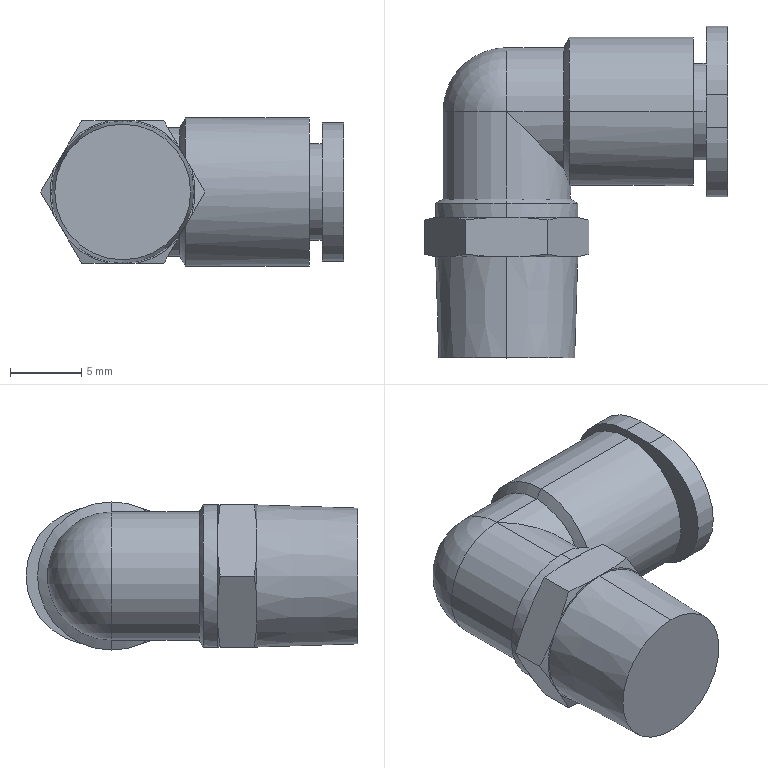Part | STEP file | KQ2L06-01GS1 | 1 solid | 55 faces | box 21.274 x 23.3 x 10.4 mm | volume 2057 mm3 | plane 20 | cone 19 | cylinder 15 | sphere 1 | commonest cylinder face diameters 9 x5 6 x2 6.8 x2 9.7 x2 10 x2 10.4 x2